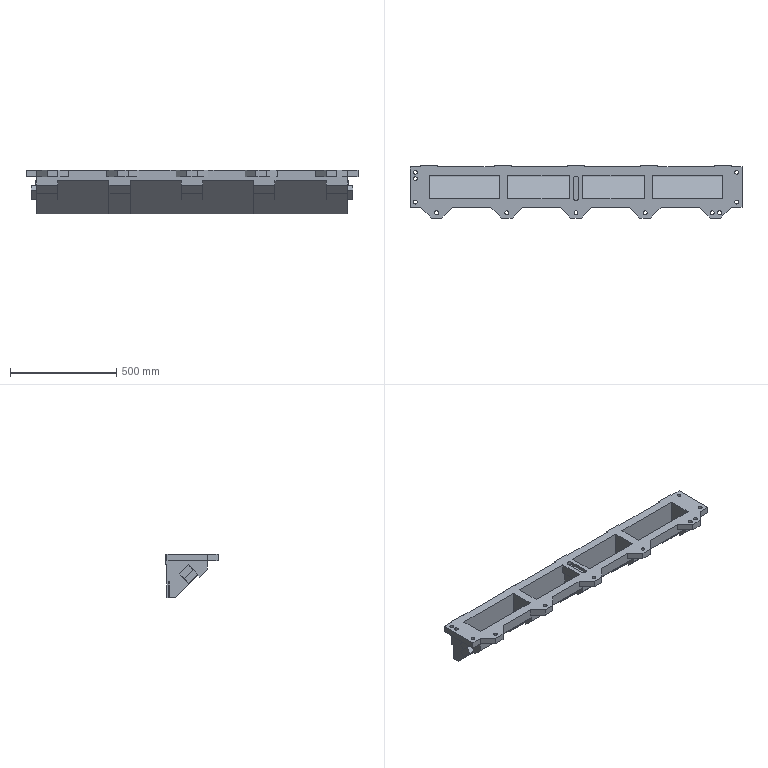Part | NX | features solid 2 | 1 solid | 181 faces | box 1560 x 245 x 205 mm | volume 28913341 mm3 | plane 151 | cylinder 30 | commonest cylinder face diameters 18 x11 26 x9 10 x8 25 x2